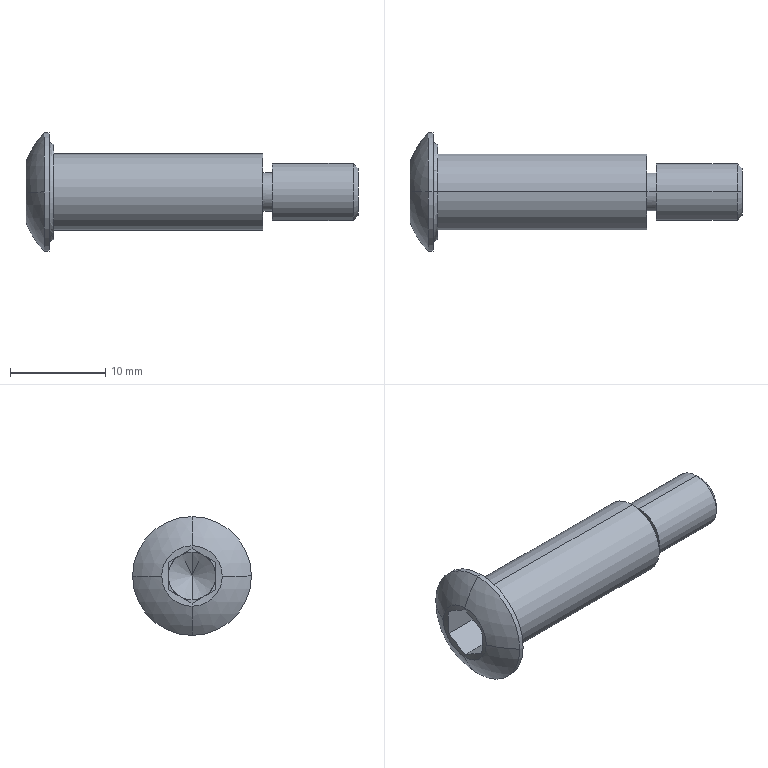Part | STEP file | 101000007750 | 1 solid | 39 faces | box 34.924 x 12.5 x 12.5 mm | volume 1534 mm3 | plane 17 | cylinder 10 | cone 6 | sphere 4 | torus 2 | commonest cylinder face diameters 4 x2 5 x2 6 x2 8 x2 12.5 x2
STEP:
#1=CARTESIAN_POINT('',(3.,0.,-5.5));
#2=VERTEX_POINT('',#1);
#3=CARTESIAN_POINT('',(3.,0.,5.5));
#4=VERTEX_POINT('',#3);
#5=CARTESIAN_POINT('',(3.,0.,0.));
#6=DIRECTION('',(-1.,0.,0.));
#7=AXIS2_PLACEMENT_3D('',#5,#6,$);
#8=CIRCLE('',#7,5.5);
#9=EDGE_CURVE('',#2,#4,#8,.T.);
#10=ORIENTED_EDGE('',*,*,#9,.F.);
#11=CARTESIAN_POINT('',(3.5,0.,-5.));
#12=VERTEX_POINT('',#11);
#13=CARTESIAN_POINT('',(3.5,0.,-5.5));
#14=DIRECTION('',(0.,1.,0.));
#15=AXIS2_PLACEMENT_3D('',#13,#14,$);
#16=CIRCLE('',#15,0.5);
#17=EDGE_CURVE('',#2,#12,#16,.T.);
#18=ORIENTED_EDGE('',*,*,#17,.T.);
#19=CARTESIAN_POINT('',(3.5,0.,5.));
#20=VERTEX_POINT('',#19);
#21=CARTESIAN_POINT('',(3.5,0.,0.));
#22=DIRECTION('',(-1.,0.,0.));
#23=AXIS2_PLACEMENT_3D('',#21,#22,$);
#24=CIRCLE('',#23,5.);
#25=EDGE_CURVE('',#12,#20,#24,.T.);
#26=ORIENTED_EDGE('',*,*,#25,.T.);
#27=CARTESIAN_POINT('',(3.5,0.,5.5));
#28=DIRECTION('',(0.,-1.,0.));
#29=AXIS2_PLACEMENT_3D('',#27,#28,$);
#30=CIRCLE('',#29,0.5);
#31=EDGE_CURVE('',#4,#20,#30,.T.);
#32=ORIENTED_EDGE('',*,*,#31,.F.);
#33=EDGE_LOOP('',(#10,#18,#26,#32));
#34=FACE_OUTER_BOUND('',#33,.T.);
#35=CARTESIAN_POINT('',(3.5,0.,0.));
#36=DIRECTION('',(-1.,0.,0.));
#37=DIRECTION('',(0.,0.,-1.));
#38=AXIS2_PLACEMENT_3D('',#35,#36,#37);
#39=TOROIDAL_SURFACE('',#38,5.5,0.5);
#40=ADVANCED_FACE('',(#34),#39,.F.);
#41=CARTESIAN_POINT('',(3.,0.,6.25));
#42=VERTEX_POINT('',#41);
#43=CARTESIAN_POINT('',(3.,0.,-6.25));
#44=VERTEX_POINT('',#43);
#45=CARTESIAN_POINT('',(3.,0.,0.));
#46=DIRECTION('',(-1.,0.,0.));
#47=AXIS2_PLACEMENT_3D('',#45,#46,$);
#48=CIRCLE('',#47,6.25);
#49=EDGE_CURVE('',#42,#44,#48,.T.);
#50=ORIENTED_EDGE('',*,*,#49,.F.);
#51=CARTESIAN_POINT('',(3.,0.,0.));
#52=DIRECTION('',(-1.,0.,0.));
#53=AXIS2_PLACEMENT_3D('',#51,#52,$);
#54=CIRCLE('',#53,6.25);
#55=EDGE_CURVE('',#44,#42,#54,.T.);
#56=ORIENTED_EDGE('',*,*,#55,.F.);
#57=EDGE_LOOP('',(#50,#56));
#58=FACE_OUTER_BOUND('',#57,.T.);
#59=CARTESIAN_POINT('',(3.,0.,0.));
#60=DIRECTION('',(-1.,0.,0.));
#61=AXIS2_PLACEMENT_3D('',#59,#60,$);
#62=CIRCLE('',#61,5.5);
#63=EDGE_CURVE('',#4,#2,#62,.T.);
#64=ORIENTED_EDGE('',*,*,#63,.T.);
#65=ORIENTED_EDGE('',*,*,#9,.T.);
#66=EDGE_LOOP('',(#64,#65));
#67=FACE_BOUND('',#66,.T.);
#68=CARTESIAN_POINT('',(3.,6.25,0.));
#69=DIRECTION('',(-1.,0.,0.));
#70=DIRECTION('',(0.,0.,1.));
#71=AXIS2_PLACEMENT_3D('',#68,#69,#70);
#72=PLANE('',#71);
#73=ADVANCED_FACE('',(#58,#67),#72,.F.);
#74=ORIENTED_EDGE('',*,*,#17,.F.);
#75=ORIENTED_EDGE('',*,*,#63,.F.);
#76=ORIENTED_EDGE('',*,*,#31,.T.);
#77=CARTESIAN_POINT('',(3.5,0.,0.));
#78=DIRECTION('',(-1.,0.,0.));
#79=AXIS2_PLACEMENT_3D('',#77,#78,$);
#80=CIRCLE('',#79,5.);
#81=EDGE_CURVE('',#20,#12,#80,.T.);
#82=ORIENTED_EDGE('',*,*,#81,.T.);
#83=EDGE_LOOP('',(#74,#75,#76,#82));
#84=FACE_OUTER_BOUND('',#83,.T.);
#85=CARTESIAN_POINT('',(3.5,0.,0.));
#86=DIRECTION('',(-1.,0.,0.));
#87=DIRECTION('',(0.,0.,1.));
#88=AXIS2_PLACEMENT_3D('',#85,#86,#87);
#89=TOROIDAL_SURFACE('',#88,5.5,0.5);
#90=ADVANCED_FACE('',(#84),#89,.F.);
#91=ORIENTED_EDGE('',*,*,#81,.F.);
#92=ORIENTED_EDGE('',*,*,#25,.F.);
#93=EDGE_LOOP('',(#91,#92));
#94=FACE_OUTER_BOUND('',#93,.T.);
#95=CARTESIAN_POINT('',(3.5,0.,4.));
#96=VERTEX_POINT('',#95);
#97=CARTESIAN_POINT('',(3.5,0.,-4.));
#98=VERTEX_POINT('',#97);
#99=CARTESIAN_POINT('',(3.5,0.,0.));
#100=DIRECTION('',(-1.,0.,0.));
#101=AXIS2_PLACEMENT_3D('',#99,#100,$);
#102=CIRCLE('',#101,4.);
#103=EDGE_CURVE('',#96,#98,#102,.T.);
#104=ORIENTED_EDGE('',*,*,#103,.T.);
#105=CARTESIAN_POINT('',(3.5,0.,0.));
#106=DIRECTION('',(-1.,0.,0.));
#107=AXIS2_PLACEMENT_3D('',#105,#106,$);
#108=CIRCLE('',#107,4.);
#109=EDGE_CURVE('',#98,#96,#108,.T.);
#110=ORIENTED_EDGE('',*,*,#109,.T.);
#111=EDGE_LOOP('',(#104,#110));
#112=FACE_BOUND('',#111,.T.);
#113=CARTESIAN_POINT('',(3.5,5.,0.));
#114=DIRECTION('',(-1.,0.,0.));
#115=DIRECTION('',(0.,0.,1.));
#116=AXIS2_PLACEMENT_3D('',#113,#114,#115);
#117=PLANE('',#116);
#118=ADVANCED_FACE('',(#94,#112),#117,.F.);
#119=ORIENTED_EDGE('',*,*,#49,.T.);
#120=CARTESIAN_POINT('',(2.5,0.,-6.25));
#121=VERTEX_POINT('',#120);
#122=CARTESIAN_POINT('',(0.,0.,-6.25));
#123=DIRECTION('',(-1.,0.,0.));
#124=VECTOR('',#123,1.);
#125=LINE('',#122,#124);
#126=EDGE_CURVE('',#44,#121,#125,.T.);
#127=ORIENTED_EDGE('',*,*,#126,.T.);
#128=CARTESIAN_POINT('',(2.5,6.25,0.));
#129=VERTEX_POINT('',#128);
#130=CARTESIAN_POINT('',(2.5,0.,0.));
#131=DIRECTION('',(-1.,0.,0.));
#132=AXIS2_PLACEMENT_3D('',#130,#131,$);
#133=CIRCLE('',#132,6.25);
#134=EDGE_CURVE('',#129,#121,#133,.T.);
#135=ORIENTED_EDGE('',*,*,#134,.F.);
#136=CARTESIAN_POINT('',(2.5,0.,6.25));
#137=VERTEX_POINT('',#136);
#138=CARTESIAN_POINT('',(2.5,0.,0.));
#139=DIRECTION('',(-1.,0.,0.));
#140=AXIS2_PLACEMENT_3D('',#138,#139,$);
#141=CIRCLE('',#140,6.25);
#142=EDGE_CURVE('',#137,#129,#141,.T.);
#143=ORIENTED_EDGE('',*,*,#142,.F.);
#144=CARTESIAN_POINT('',(0.,0.,6.25));
#145=DIRECTION('',(-1.,0.,0.));
#146=VECTOR('',#145,1.);
#147=LINE('',#144,#146);
#148=EDGE_CURVE('',#42,#137,#147,.T.);
#149=ORIENTED_EDGE('',*,*,#148,.F.);
#150=EDGE_LOOP('',(#119,#127,#135,#143,#149));
#151=FACE_OUTER_BOUND('',#150,.T.);
#152=CARTESIAN_POINT('',(0.,0.,0.));
#153=DIRECTION('',(-1.,0.,0.));
#154=DIRECTION('',(0.,0.,1.));
#155=AXIS2_PLACEMENT_3D('',#152,#153,#154);
#156=CYLINDRICAL_SURFACE('',#155,6.25);
#157=ADVANCED_FACE('',(#151),#156,.T.);
#158=ORIENTED_EDGE('',*,*,#126,.F.);
#159=ORIENTED_EDGE('',*,*,#55,.T.);
#160=ORIENTED_EDGE('',*,*,#148,.T.);
#161=CARTESIAN_POINT('',(2.5,-6.25,0.));
#162=VERTEX_POINT('',#161);
#163=CARTESIAN_POINT('',(2.5,0.,0.));
#164=DIRECTION('',(-1.,0.,0.));
#165=AXIS2_PLACEMENT_3D('',#163,#164,$);
#166=CIRCLE('',#165,6.25);
#167=EDGE_CURVE('',#162,#137,#166,.T.);
#168=ORIENTED_EDGE('',*,*,#167,.F.);
#169=CARTESIAN_POINT('',(2.5,0.,0.));
#170=DIRECTION('',(-1.,0.,0.));
#171=AXIS2_PLACEMENT_3D('',#169,#170,$);
#172=CIRCLE('',#171,6.25);
#173=EDGE_CURVE('',#121,#162,#172,.T.);
#174=ORIENTED_EDGE('',*,*,#173,.F.);
#175=EDGE_LOOP('',(#158,#159,#160,#168,#174));
#176=FACE_OUTER_BOUND('',#175,.T.);
#177=CARTESIAN_POINT('',(0.,0.,0.));
#178=DIRECTION('',(-1.,0.,0.));
#179=DIRECTION('',(0.,0.,-1.));
#180=AXIS2_PLACEMENT_3D('',#177,#178,#179);
#181=CYLINDRICAL_SURFACE('',#180,6.25);
#182=ADVANCED_FACE('',(#176),#181,.T.);
#183=CARTESIAN_POINT('',(25.5,0.,4.));
#184=VERTEX_POINT('',#183);
#185=CARTESIAN_POINT('',(25.5,0.,-4.));
#186=VERTEX_POINT('',#185);
#187=CARTESIAN_POINT('',(25.5,0.,0.));
#188=DIRECTION('',(-1.,0.,0.));
#189=AXIS2_PLACEMENT_3D('',#187,#188,$);
#190=CIRCLE('',#189,4.);
#191=EDGE_CURVE('',#184,#186,#190,.T.);
#192=ORIENTED_EDGE('',*,*,#191,.T.);
#193=CARTESIAN_POINT('',(0.,0.,-4.));
#194=DIRECTION('',(-1.,0.,0.));
#195=VECTOR('',#194,1.);
#196=LINE('',#193,#195);
#197=EDGE_CURVE('',#186,#98,#196,.T.);
#198=ORIENTED_EDGE('',*,*,#197,.T.);
#199=ORIENTED_EDGE('',*,*,#103,.F.);
#200=CARTESIAN_POINT('',(0.,0.,4.));
#201=DIRECTION('',(-1.,0.,0.));
#202=VECTOR('',#201,1.);
#203=LINE('',#200,#202);
#204=EDGE_CURVE('',#184,#96,#203,.T.);
#205=ORIENTED_EDGE('',*,*,#204,.F.);
#206=EDGE_LOOP('',(#192,#198,#199,#205));
#207=FACE_OUTER_BOUND('',#206,.T.);
#208=CARTESIAN_POINT('',(0.,0.,0.));
#209=DIRECTION('',(-1.,0.,0.));
#210=DIRECTION('',(0.,0.,1.));
#211=AXIS2_PLACEMENT_3D('',#208,#209,#210);
#212=CYLINDRICAL_SURFACE('',#211,4.);
#213=ADVANCED_FACE('',(#207),#212,.T.);
#214=ORIENTED_EDGE('',*,*,#197,.F.);
#215=CARTESIAN_POINT('',(25.5,0.,0.));
#216=DIRECTION('',(-1.,0.,0.));
#217=AXIS2_PLACEMENT_3D('',#215,#216,$);
#218=CIRCLE('',#217,4.);
#219=EDGE_CURVE('',#186,#184,#218,.T.);
#220=ORIENTED_EDGE('',*,*,#219,.T.);
#221=ORIENTED_EDGE('',*,*,#204,.T.);
#222=ORIENTED_EDGE('',*,*,#109,.F.);
#223=EDGE_LOOP('',(#214,#220,#221,#222));
#224=FACE_OUTER_BOUND('',#223,.T.);
#225=CARTESIAN_POINT('',(0.,0.,0.));
#226=DIRECTION('',(-1.,0.,0.));
#227=DIRECTION('',(0.,0.,-1.));
#228=AXIS2_PLACEMENT_3D('',#225,#226,#227);
#229=CYLINDRICAL_SURFACE('',#228,4.);
#230=ADVANCED_FACE('',(#224),#229,.T.);
#231=CARTESIAN_POINT('',(0.5761,0.,-3.18));
#232=VERTEX_POINT('',#231);
#233=CARTESIAN_POINT('',(9.062,0.,0.));
#234=DIRECTION('',(0.,-1.,0.));
#235=AXIS2_PLACEMENT_3D('',#233,#234,$);
#236=CIRCLE('',#235,9.062);
#237=EDGE_CURVE('',#232,#121,#236,.T.);
#238=ORIENTED_EDGE('',*,*,#237,.F.);
#239=CARTESIAN_POINT('',(0.5761,3.18,0.));
#240=VERTEX_POINT('',#239);
#241=CARTESIAN_POINT('',(0.5761,3.18,0.));
#242=CARTESIAN_POINT('',(0.5761,3.18,-1.011));
#243=CARTESIAN_POINT('',(0.5761,2.782,-2.028));
#244=CARTESIAN_POINT('',(0.5761,1.955,-2.812));
#245=CARTESIAN_POINT('',(0.5761,0.9776,-3.18));
#246=CARTESIAN_POINT('',(0.5761,0.,-3.18));
#247=B_SPLINE_CURVE_WITH_KNOTS('',5,(#241,#242,#243,#244,#245,#246),.UNSPECIFIED.,.F.,.U.,(6,6),(0.,7.151),.UNSPECIFIED.);
#248=EDGE_CURVE('',#240,#232,#247,.T.);
#249=ORIENTED_EDGE('',*,*,#248,.F.);
#250=CARTESIAN_POINT('',(9.062,0.,0.));
#251=DIRECTION('',(0.,0.,-1.));
#252=AXIS2_PLACEMENT_3D('',#250,#251,$);
#253=CIRCLE('',#252,9.062);
#254=EDGE_CURVE('',#129,#240,#253,.F.);
#255=ORIENTED_EDGE('',*,*,#254,.F.);
#256=ORIENTED_EDGE('',*,*,#134,.T.);
#257=EDGE_LOOP('',(#238,#249,#255,#256));
#258=FACE_OUTER_BOUND('',#257,.T.);
#259=CARTESIAN_POINT('',(9.062,0.,0.));
#260=DIRECTION('',(0.,0.,-1.));
#261=DIRECTION('',(-1.,0.,0.));
#262=AXIS2_PLACEMENT_3D('',#259,#260,#261);
#263=SPHERICAL_SURFACE('',#262,9.062);
#264=ADVANCED_FACE('',(#258),#263,.T.);
#265=CARTESIAN_POINT('',(0.5761,0.,3.18));
#266=VERTEX_POINT('',#265);
#267=CARTESIAN_POINT('',(9.062,0.,0.));
#268=DIRECTION('',(0.,-1.,0.));
#269=AXIS2_PLACEMENT_3D('',#267,#268,$);
#270=CIRCLE('',#269,9.062);
#271=EDGE_CURVE('',#137,#266,#270,.T.);
#272=ORIENTED_EDGE('',*,*,#271,.F.);
#273=ORIENTED_EDGE('',*,*,#142,.T.);
#274=ORIENTED_EDGE('',*,*,#254,.T.);
#275=CARTESIAN_POINT('',(0.5761,0.,3.18));
#276=CARTESIAN_POINT('',(0.5761,0.9776,3.18));
#277=CARTESIAN_POINT('',(0.5761,1.955,2.812));
#278=CARTESIAN_POINT('',(0.5761,2.782,2.028));
#279=CARTESIAN_POINT('',(0.5761,3.18,1.011));
#280=CARTESIAN_POINT('',(0.5761,3.18,0.));
#281=B_SPLINE_CURVE_WITH_KNOTS('',5,(#275,#276,#277,#278,#279,#280),.UNSPECIFIED.,.F.,.U.,(6,6),(0.,7.151),.UNSPECIFIED.);
#282=EDGE_CURVE('',#266,#240,#281,.T.);
#283=ORIENTED_EDGE('',*,*,#282,.F.);
#284=EDGE_LOOP('',(#272,#273,#274,#283));
#285=FACE_OUTER_BOUND('',#284,.T.);
#286=CARTESIAN_POINT('',(9.062,0.,0.));
#287=DIRECTION('',(0.,0.,-1.));
#288=DIRECTION('',(-1.,0.,0.));
#289=AXIS2_PLACEMENT_3D('',#286,#287,#288);
#290=SPHERICAL_SURFACE('',#289,9.062);
#291=ADVANCED_FACE('',(#285),#290,.T.);
#292=ORIENTED_EDGE('',*,*,#271,.T.);
#293=CARTESIAN_POINT('',(0.5761,-3.18,0.));
#294=VERTEX_POINT('',#293);
#295=CARTESIAN_POINT('',(0.5761,-3.18,0.));
#296=CARTESIAN_POINT('',(0.5761,-3.18,1.011));
#297=CARTESIAN_POINT('',(0.5761,-2.782,2.028));
#298=CARTESIAN_POINT('',(0.5761,-1.955,2.812));
#299=CARTESIAN_POINT('',(0.5761,-0.9776,3.18));
#300=CARTESIAN_POINT('',(0.5761,0.,3.18));
#301=B_SPLINE_CURVE_WITH_KNOTS('',5,(#295,#296,#297,#298,#299,#300),.UNSPECIFIED.,.F.,.U.,(6,6),(0.,7.151),.UNSPECIFIED.);
#302=EDGE_CURVE('',#294,#266,#301,.T.);
#303=ORIENTED_EDGE('',*,*,#302,.F.);
#304=CARTESIAN_POINT('',(9.062,0.,0.));
#305=DIRECTION('',(0.,0.,-1.));
#306=AXIS2_PLACEMENT_3D('',#304,#305,$);
#307=CIRCLE('',#306,9.062);
#308=EDGE_CURVE('',#162,#294,#307,.T.);
#309=ORIENTED_EDGE('',*,*,#308,.F.);
#310=ORIENTED_EDGE('',*,*,#167,.T.);
#311=EDGE_LOOP('',(#292,#303,#309,#310));
#312=FACE_OUTER_BOUND('',#311,.T.);
#313=CARTESIAN_POINT('',(9.062,0.,0.));
#314=DIRECTION('',(0.,0.,-1.));
#315=DIRECTION('',(0.,-1.,0.));
#316=AXIS2_PLACEMENT_3D('',#313,#314,#315);
#317=SPHERICAL_SURFACE('',#316,9.062);
#318=ADVANCED_FACE('',(#312),#317,.T.);
#319=ORIENTED_EDGE('',*,*,#237,.T.);
#320=ORIENTED_EDGE('',*,*,#173,.T.);
#321=ORIENTED_EDGE('',*,*,#308,.T.);
#322=CARTESIAN_POINT('',(0.5761,0.,-3.18));
#323=CARTESIAN_POINT('',(0.5761,-0.9776,-3.18));
#324=CARTESIAN_POINT('',(0.5761,-1.955,-2.812));
#325=CARTESIAN_POINT('',(0.5761,-2.782,-2.028));
#326=CARTESIAN_POINT('',(0.5761,-3.18,-1.011));
#327=CARTESIAN_POINT('',(0.5761,-3.18,0.));
#328=B_SPLINE_CURVE_WITH_KNOTS('',5,(#322,#323,#324,#325,#326,#327),.UNSPECIFIED.,.F.,.U.,(6,6),(0.,7.151),.UNSPECIFIED.);
#329=EDGE_CURVE('',#232,#294,#328,.T.);
#330=ORIENTED_EDGE('',*,*,#329,.F.);
#331=EDGE_LOOP('',(#319,#320,#321,#330));
#332=FACE_OUTER_BOUND('',#331,.T.);
#333=CARTESIAN_POINT('',(9.062,0.,0.));
#334=DIRECTION('',(0.,0.,-1.));
#335=DIRECTION('',(0.,-1.,0.));
#336=AXIS2_PLACEMENT_3D('',#333,#334,#335);
#337=SPHERICAL_SURFACE('',#336,9.062);
#338=ADVANCED_FACE('',(#332),#337,.T.);
#339=ORIENTED_EDGE('',*,*,#191,.F.);
#340=ORIENTED_EDGE('',*,*,#219,.F.);
#341=EDGE_LOOP('',(#339,#340));
#342=FACE_OUTER_BOUND('',#341,.T.);
#343=CARTESIAN_POINT('',(25.5,0.,-2.));
#344=VERTEX_POINT('',#343);
#345=CARTESIAN_POINT('',(25.5,0.,2.));
#346=VERTEX_POINT('',#345);
#347=CARTESIAN_POINT('',(25.5,0.,-2.));
#348=CARTESIAN_POINT('',(25.5,0.2078,-2.));
#349=CARTESIAN_POINT('',(25.5,0.4157,-1.973));
#350=CARTESIAN_POINT('',(25.5,0.6189,-1.919));
#351=CARTESIAN_POINT('',(25.5,1.006,-1.759));
#352=CARTESIAN_POINT('',(25.5,1.341,-1.506));
#353=CARTESIAN_POINT('',(25.5,1.49,-1.358));
#354=CARTESIAN_POINT('',(25.5,1.747,-1.027));
#355=CARTESIAN_POINT('',(25.5,1.911,-0.6418));
#356=CARTESIAN_POINT('',(25.5,1.968,-0.4392));
#357=CARTESIAN_POINT('',(25.5,2.027,-0.02422));
#358=CARTESIAN_POINT('',(25.5,1.978,0.3921));
#359=CARTESIAN_POINT('',(25.5,1.926,0.5959));
#360=CARTESIAN_POINT('',(25.5,1.771,0.9854));
#361=CARTESIAN_POINT('',(25.5,1.522,1.322));
#362=CARTESIAN_POINT('',(25.5,1.376,1.474));
#363=CARTESIAN_POINT('',(25.5,1.048,1.735));
#364=CARTESIAN_POINT('',(25.5,0.6646,1.904));
#365=CARTESIAN_POINT('',(25.5,0.4627,1.963));
#366=CARTESIAN_POINT('',(25.5,0.2461,1.996));
#367=CARTESIAN_POINT('',(25.5,0.02868,2.));
#368=CARTESIAN_POINT('',(25.5,0.01912,2.));
#369=CARTESIAN_POINT('',(25.5,0.00956,2.));
#370=CARTESIAN_POINT('',(25.5,0.,2.));
#371=B_SPLINE_CURVE_WITH_KNOTS('',5,(#347,#348,#349,#350,#351,#352,#353,#354,#355,#356,#357,#358,#359,#360,#361,#362,#363,#364,#365,#366,#367,#368,#369,#370),.UNSPECIFIED.,.F.,.U.,(6,3,3,3,3,3,3,6),(0.,1.47,2.939,4.409,5.879,7.348,8.818,8.886),.UNSPECIFIED.);
#372=EDGE_CURVE('',#344,#346,#371,.T.);
#373=ORIENTED_EDGE('',*,*,#372,.F.);
#374=CARTESIAN_POINT('',(25.5,0.,2.));
#375=CARTESIAN_POINT('',(25.5,-0.2078,2.));
#376=CARTESIAN_POINT('',(25.5,-0.4157,1.973));
#377=CARTESIAN_POINT('',(25.5,-0.6189,1.919));
#378=CARTESIAN_POINT('',(25.5,-1.006,1.759));
#379=CARTESIAN_POINT('',(25.5,-1.341,1.506));
#380=CARTESIAN_POINT('',(25.5,-1.49,1.358));
#381=CARTESIAN_POINT('',(25.5,-1.747,1.027));
#382=CARTESIAN_POINT('',(25.5,-1.911,0.6418));
#383=CARTESIAN_POINT('',(25.5,-1.968,0.4392));
#384=CARTESIAN_POINT('',(25.5,-2.027,0.02422));
#385=CARTESIAN_POINT('',(25.5,-1.978,-0.3921));
#386=CARTESIAN_POINT('',(25.5,-1.926,-0.5959));
#387=CARTESIAN_POINT('',(25.5,-1.771,-0.9854));
#388=CARTESIAN_POINT('',(25.5,-1.522,-1.322));
#389=CARTESIAN_POINT('',(25.5,-1.376,-1.474));
#390=CARTESIAN_POINT('',(25.5,-1.048,-1.735));
#391=CARTESIAN_POINT('',(25.5,-0.6646,-1.904));
#392=CARTESIAN_POINT('',(25.5,-0.4627,-1.963));
#393=CARTESIAN_POINT('',(25.5,-0.2461,-1.996));
#394=CARTESIAN_POINT('',(25.5,-0.02868,-2.));
#395=CARTESIAN_POINT('',(25.5,-0.01912,-2.));
#396=CARTESIAN_POINT('',(25.5,-0.00956,-2.));
#397=CARTESIAN_POINT('',(25.5,0.,-2.));
#398=B_SPLINE_CURVE_WITH_KNOTS('',5,(#374,#375,#376,#377,#378,#379,#380,#381,#382,#383,#384,#385,#386,#387,#388,#389,#390,#391,#392,#393,#394,#395,#396,#397),.UNSPECIFIED.,.F.,.U.,(6,3,3,3,3,3,3,6),(0.,1.47,2.939,4.409,5.879,7.348,8.818,8.886),.UNSPECIFIED.);
#399=EDGE_CURVE('',#346,#344,#398,.T.);
#400=ORIENTED_EDGE('',*,*,#399,.F.);
#401=EDGE_LOOP('',(#373,#400));
#402=FACE_BOUND('',#401,.T.);
#403=CARTESIAN_POINT('',(25.5,4.,0.));
#404=DIRECTION('',(-1.,0.,0.));
#405=DIRECTION('',(0.,0.,1.));
#406=AXIS2_PLACEMENT_3D('',#403,#404,#405);
#407=PLANE('',#406);
#408=ADVANCED_FACE('',(#342,#402),#407,.F.);
#409=CARTESIAN_POINT('',(0.6151,0.,-2.887));
#410=VERTEX_POINT('',#409);
#411=CARTESIAN_POINT('',(-66580.86,0.,-499363.95));
#412=DIRECTION('',(-0.1322,0.,-0.9912));
#413=VECTOR('',#412,1.);
#414=LINE('',#411,#413);
#415=EDGE_CURVE('',#410,#232,#414,.T.);
#416=ORIENTED_EDGE('',*,*,#415,.F.);
#417=CARTESIAN_POINT('',(0.6151,2.5,-1.443));
#418=VERTEX_POINT('',#417);
#419=CARTESIAN_POINT('',(0.6151,2.5,-1.443));
#420=CARTESIAN_POINT('',(0.6617,1.895,-1.793));
#421=CARTESIAN_POINT('',(0.6741,1.472,-2.037));
#422=CARTESIAN_POINT('',(0.6743,1.029,-2.293));
#423=CARTESIAN_POINT('',(0.6617,0.6048,-2.538));
#424=CARTESIAN_POINT('',(0.6151,0.,-2.887));
#425=B_SPLINE_CURVE_WITH_KNOTS('',5,(#419,#420,#421,#422,#423,#424),.UNSPECIFIED.,.F.,.U.,(6,6),(0.,104.832),.UNSPECIFIED.);
#426=EDGE_CURVE('',#418,#410,#425,.T.);
#427=ORIENTED_EDGE('',*,*,#426,.F.);
#428=CARTESIAN_POINT('',(0.6151,2.5,1.443));
#429=VERTEX_POINT('',#428);
#430=CARTESIAN_POINT('',(0.6151,2.5,1.443));
#431=CARTESIAN_POINT('',(0.6617,2.5,0.745));
#432=CARTESIAN_POINT('',(0.6742,2.5,0.2567));
#433=CARTESIAN_POINT('',(0.6743,2.5,-0.2555));
#434=CARTESIAN_POINT('',(0.6617,2.5,-0.745));
#435=CARTESIAN_POINT('',(0.6151,2.5,-1.443));
#436=B_SPLINE_CURVE_WITH_KNOTS('',5,(#430,#431,#432,#433,#434,#435),.UNSPECIFIED.,.F.,.U.,(6,6),(0.,104.832),.UNSPECIFIED.);
#437=EDGE_CURVE('',#429,#418,#436,.T.);
#438=ORIENTED_EDGE('',*,*,#437,.F.);
#439=CARTESIAN_POINT('',(0.6151,0.,2.887));
#440=VERTEX_POINT('',#439);
#441=CARTESIAN_POINT('',(0.6151,0.,2.887));
#442=CARTESIAN_POINT('',(0.6617,0.6048,2.538));
#443=CARTESIAN_POINT('',(0.6741,1.028,2.293));
#444=CARTESIAN_POINT('',(0.6743,1.471,2.037));
#445=CARTESIAN_POINT('',(0.6617,1.895,1.793));
#446=CARTESIAN_POINT('',(0.6151,2.5,1.443));
#447=B_SPLINE_CURVE_WITH_KNOTS('',5,(#441,#442,#443,#444,#445,#446),.UNSPECIFIED.,.F.,.U.,(6,6),(0.,104.832),.UNSPECIFIED.);
#448=EDGE_CURVE('',#440,#429,#447,.T.);
#449=ORIENTED_EDGE('',*,*,#448,.F.);
#450=CARTESIAN_POINT('',(-66580.86,0.,499363.95));
#451=DIRECTION('',(-0.1322,0.,0.9912));
#452=VECTOR('',#451,1.);
#453=LINE('',#450,#452);
#454=EDGE_CURVE('',#440,#266,#453,.T.);
#455=ORIENTED_EDGE('',*,*,#454,.T.);
#456=ORIENTED_EDGE('',*,*,#282,.T.);
#457=ORIENTED_EDGE('',*,*,#248,.T.);
#458=EDGE_LOOP('',(#416,#427,#438,#449,#455,#456,#457));
#459=FACE_OUTER_BOUND('',#458,.T.);
#460=CARTESIAN_POINT('',(-999.,0.,0.));
#461=DIRECTION('',(-1.,0.,0.));
#462=DIRECTION('',(0.,0.,1.));
#463=AXIS2_PLACEMENT_3D('',#460,#461,#462);
#464=CONICAL_SURFACE('',#463,7500.,1.438);
#465=ADVANCED_FACE('',(#459),#464,.F.);
#466=CARTESIAN_POINT('',(0.6151,-2.5,-1.443));
#467=VERTEX_POINT('',#466);
#468=CARTESIAN_POINT('',(0.6151,0.,-2.887));
#469=CARTESIAN_POINT('',(0.6617,-0.6048,-2.538));
#470=CARTESIAN_POINT('',(0.6741,-1.028,-2.293));
#471=CARTESIAN_POINT('',(0.6743,-1.471,-2.037));
#472=CARTESIAN_POINT('',(0.6617,-1.895,-1.793));
#473=CARTESIAN_POINT('',(0.6151,-2.5,-1.443));
#474=B_SPLINE_CURVE_WITH_KNOTS('',5,(#468,#469,#470,#471,#472,#473),.UNSPECIFIED.,.F.,.U.,(6,6),(0.,104.832),.UNSPECIFIED.);
#475=EDGE_CURVE('',#410,#467,#474,.T.);
#476=ORIENTED_EDGE('',*,*,#475,.F.);
#477=ORIENTED_EDGE('',*,*,#415,.T.);
#478=ORIENTED_EDGE('',*,*,#329,.T.);
#479=ORIENTED_EDGE('',*,*,#302,.T.);
#480=ORIENTED_EDGE('',*,*,#454,.F.);
#481=CARTESIAN_POINT('',(0.6151,-2.5,1.443));
#482=VERTEX_POINT('',#481);
#483=CARTESIAN_POINT('',(0.6151,-2.5,1.443));
#484=CARTESIAN_POINT('',(0.6617,-1.895,1.793));
#485=CARTESIAN_POINT('',(0.6741,-1.472,2.037));
#486=CARTESIAN_POINT('',(0.6743,-1.029,2.293));
#487=CARTESIAN_POINT('',(0.6617,-0.6048,2.538));
#488=CARTESIAN_POINT('',(0.6151,0.,2.887));
#489=B_SPLINE_CURVE_WITH_KNOTS('',5,(#483,#484,#485,#486,#487,#488),.UNSPECIFIED.,.F.,.U.,(6,6),(0.,104.832),.UNSPECIFIED.);
#490=EDGE_CURVE('',#482,#440,#489,.T.);
#491=ORIENTED_EDGE('',*,*,#490,.F.);
#492=CARTESIAN_POINT('',(0.6151,-2.5,-1.443));
#493=CARTESIAN_POINT('',(0.6617,-2.5,-0.745));
#494=CARTESIAN_POINT('',(0.6741,-2.5,-0.2567));
#495=CARTESIAN_POINT('',(0.6743,-2.5,0.2555));
#496=CARTESIAN_POINT('',(0.6617,-2.5,0.745));
#497=CARTESIAN_POINT('',(0.6151,-2.5,1.443));
#498=B_SPLINE_CURVE_WITH_KNOTS('',5,(#492,#493,#494,#495,#496,#497),.UNSPECIFIED.,.F.,.U.,(6,6),(0.,104.833),.UNSPECIFIED.);
#499=EDGE_CURVE('',#467,#482,#498,.T.);
#500=ORIENTED_EDGE('',*,*,#499,.F.);
#501=EDGE_LOOP('',(#476,#477,#478,#479,#480,#491,#500));
#502=FACE_OUTER_BOUND('',#501,.T.);
#503=CARTESIAN_POINT('',(-999.,0.,0.));
#504=DIRECTION('',(-1.,0.,0.));
#505=DIRECTION('',(0.,0.,-1.));
#506=AXIS2_PLACEMENT_3D('',#503,#504,#505);
#507=CONICAL_SURFACE('',#506,7500.,1.438);
#508=ADVANCED_FACE('',(#502),#507,.F.);
#509=ORIENTED_EDGE('',*,*,#372,.T.);
#510=CARTESIAN_POINT('',(26.5,0.,2.));
#511=VERTEX_POINT('',#510);
#512=CARTESIAN_POINT('',(35.,0.,2.));
#513=DIRECTION('',(1.,0.,0.));
#514=VECTOR('',#513,1.);
#515=LINE('',#512,#514);
#516=EDGE_CURVE('',#346,#511,#515,.T.);
#517=ORIENTED_EDGE('',*,*,#516,.T.);
#518=CARTESIAN_POINT('',(26.5,0.,-2.));
#519=VERTEX_POINT('',#518);
#520=CARTESIAN_POINT('',(26.5,0.,0.));
#521=DIRECTION('',(1.,0.,0.));
#522=AXIS2_PLACEMENT_3D('',#520,#521,$);
#523=CIRCLE('',#522,2.);
#524=EDGE_CURVE('',#519,#511,#523,.T.);
#525=ORIENTED_EDGE('',*,*,#524,.F.);
#526=CARTESIAN_POINT('',(35.,0.,-2.));
#527=DIRECTION('',(1.,0.,0.));
#528=VECTOR('',#527,1.);
#529=LINE('',#526,#528);
#530=EDGE_CURVE('',#344,#519,#529,.T.);
#531=ORIENTED_EDGE('',*,*,#530,.F.);
#532=EDGE_LOOP('',(#509,#517,#525,#531));
#533=FACE_OUTER_BOUND('',#532,.T.);
#534=CARTESIAN_POINT('',(35.,0.,0.));
#535=DIRECTION('',(1.,0.,0.));
#536=DIRECTION('',(0.,0.,-1.));
#537=AXIS2_PLACEMENT_3D('',#534,#535,#536);
#538=CYLINDRICAL_SURFACE('',#537,2.);
#539=ADVANCED_FACE('',(#533),#538,.T.);
#540=ORIENTED_EDGE('',*,*,#516,.F.);
#541=ORIENTED_EDGE('',*,*,#399,.T.);
#542=ORIENTED_EDGE('',*,*,#530,.T.);
#543=CARTESIAN_POINT('',(26.5,0.,0.));
#544=DIRECTION('',(1.,0.,0.));
#545=AXIS2_PLACEMENT_3D('',#543,#544,$);
#546=CIRCLE('',#545,2.);
#547=EDGE_CURVE('',#511,#519,#546,.T.);
#548=ORIENTED_EDGE('',*,*,#547,.F.);
#549=EDGE_LOOP('',(#540,#541,#542,#548));
#550=FACE_OUTER_BOUND('',#549,.T.);
#551=CARTESIAN_POINT('',(35.,0.,0.));
#552=DIRECTION('',(1.,0.,0.));
#553=DIRECTION('',(0.,0.,1.));
#554=AXIS2_PLACEMENT_3D('',#551,#552,#553);
#555=CYLINDRICAL_SURFACE('',#554,2.);
#556=ADVANCED_FACE('',(#550),#555,.T.);
#557=CARTESIAN_POINT('',(4.3,0.,-2.887));
#558=VERTEX_POINT('',#557);
#559=CARTESIAN_POINT('',(4.3,1.25,-2.165));
#560=VERTEX_POINT('',#559);
#561=CARTESIAN_POINT('',(4.3,0.625,-2.526));
#562=DIRECTION('',(0.,0.866,0.5));
#563=VECTOR('',#562,1.);
#564=LINE('',#561,#563);
#565=EDGE_CURVE('',#558,#560,#564,.T.);
#566=ORIENTED_EDGE('',*,*,#565,.T.);
#567=CARTESIAN_POINT('',(4.3,2.5,-1.443));
#568=VERTEX_POINT('',#567);
#569=CARTESIAN_POINT('',(4.3,1.875,-1.804));
#570=DIRECTION('',(0.,0.866,0.5));
#571=VECTOR('',#570,1.);
#572=LINE('',#569,#571);
#573=EDGE_CURVE('',#560,#568,#572,.T.);
#574=ORIENTED_EDGE('',*,*,#573,.T.);
#575=CARTESIAN_POINT('',(2.458,2.5,-1.443));
#576=DIRECTION('',(-1.,0.,0.));
#577=VECTOR('',#576,1.);
#578=LINE('',#575,#577);
#579=EDGE_CURVE('',#568,#418,#578,.T.);
#580=ORIENTED_EDGE('',*,*,#579,.T.);
#581=ORIENTED_EDGE('',*,*,#426,.T.);
#582=CARTESIAN_POINT('',(2.458,0.,-2.887));
#583=DIRECTION('',(-1.,0.,0.));
#584=VECTOR('',#583,1.);
#585=LINE('',#582,#584);
#586=EDGE_CURVE('',#558,#410,#585,.T.);
#587=ORIENTED_EDGE('',*,*,#586,.F.);
#588=EDGE_LOOP('',(#566,#574,#580,#581,#587));
#589=FACE_OUTER_BOUND('',#588,.T.);
#590=CARTESIAN_POINT('',(4.3,0.,-2.887));
#591=DIRECTION('',(0.,-0.5,0.866));
#592=DIRECTION('',(0.,-0.866,-0.5));
#593=AXIS2_PLACEMENT_3D('',#590,#591,#592);
#594=PLANE('',#593);
#595=ADVANCED_FACE('',(#589),#594,.T.);
#596=CARTESIAN_POINT('',(4.3,2.5,0.));
#597=VERTEX_POINT('',#596);
#598=CARTESIAN_POINT('',(4.3,2.5,-0.7217));
#599=DIRECTION('',(0.,0.,1.));
#600=VECTOR('',#599,1.);
#601=LINE('',#598,#600);
#602=EDGE_CURVE('',#568,#597,#601,.T.);
#603=ORIENTED_EDGE('',*,*,#602,.T.);
#604=CARTESIAN_POINT('',(4.3,2.5,1.443));
#605=VERTEX_POINT('',#604);
#606=CARTESIAN_POINT('',(4.3,2.5,0.7217));
#607=DIRECTION('',(0.,0.,1.));
#608=VECTOR('',#607,1.);
#609=LINE('',#606,#608);
#610=EDGE_CURVE('',#597,#605,#609,.T.);
#611=ORIENTED_EDGE('',*,*,#610,.T.);
#612=CARTESIAN_POINT('',(2.458,2.5,1.443));
#613=DIRECTION('',(-1.,0.,0.));
#614=VECTOR('',#613,1.);
#615=LINE('',#612,#614);
#616=EDGE_CURVE('',#605,#429,#615,.T.);
#617=ORIENTED_EDGE('',*,*,#616,.T.);
#618=ORIENTED_EDGE('',*,*,#437,.T.);
#619=ORIENTED_EDGE('',*,*,#579,.F.);
#620=EDGE_LOOP('',(#603,#611,#617,#618,#619));
#621=FACE_OUTER_BOUND('',#620,.T.);
#622=CARTESIAN_POINT('',(4.3,2.5,-1.443));
#623=DIRECTION('',(0.,-1.,0.));
#624=DIRECTION('',(0.,0.,-1.));
#625=AXIS2_PLACEMENT_3D('',#622,#623,#624);
#626=PLANE('',#625);
#627=ADVANCED_FACE('',(#621),#626,.T.);
#628=CARTESIAN_POINT('',(4.3,1.25,2.165));
#629=VERTEX_POINT('',#628);
#630=CARTESIAN_POINT('',(4.3,1.875,1.804));
#631=DIRECTION('',(0.,-0.866,0.5));
#632=VECTOR('',#631,1.);
#633=LINE('',#630,#632);
#634=EDGE_CURVE('',#605,#629,#633,.T.);
#635=ORIENTED_EDGE('',*,*,#634,.T.);
#636=CARTESIAN_POINT('',(4.3,0.,2.887));
#637=VERTEX_POINT('',#636);
#638=CARTESIAN_POINT('',(4.3,0.625,2.526));
#639=DIRECTION('',(0.,-0.866,0.5));
#640=VECTOR('',#639,1.);
#641=LINE('',#638,#640);
#642=EDGE_CURVE('',#629,#637,#641,.T.);
#643=ORIENTED_EDGE('',*,*,#642,.T.);
#644=CARTESIAN_POINT('',(2.458,0.,2.887));
#645=DIRECTION('',(-1.,0.,0.));
#646=VECTOR('',#645,1.);
#647=LINE('',#644,#646);
#648=EDGE_CURVE('',#637,#440,#647,.T.);
#649=ORIENTED_EDGE('',*,*,#648,.T.);
#650=ORIENTED_EDGE('',*,*,#448,.T.);
#651=ORIENTED_EDGE('',*,*,#616,.F.);
#652=EDGE_LOOP('',(#635,#643,#649,#650,#651));
#653=FACE_OUTER_BOUND('',#652,.T.);
#654=CARTESIAN_POINT('',(4.3,2.5,1.443));
#655=DIRECTION('',(0.,-0.5,-0.866));
#656=DIRECTION('',(0.,0.866,-0.5));
#657=AXIS2_PLACEMENT_3D('',#654,#655,#656);
#658=PLANE('',#657);
#659=ADVANCED_FACE('',(#653),#658,.T.);
#660=CARTESIAN_POINT('',(4.3,-2.5,-1.443));
#661=VERTEX_POINT('',#660);
#662=CARTESIAN_POINT('',(4.3,-1.25,-2.165));
#663=VERTEX_POINT('',#662);
#664=CARTESIAN_POINT('',(4.3,-1.875,-1.804));
#665=DIRECTION('',(0.,0.866,-0.5));
#666=VECTOR('',#665,1.);
#667=LINE('',#664,#666);
#668=EDGE_CURVE('',#661,#663,#667,.T.);
#669=ORIENTED_EDGE('',*,*,#668,.T.);
#670=CARTESIAN_POINT('',(4.3,-0.625,-2.526));
#671=DIRECTION('',(0.,0.866,-0.5));
#672=VECTOR('',#671,1.);
#673=LINE('',#670,#672);
#674=EDGE_CURVE('',#663,#558,#673,.T.);
#675=ORIENTED_EDGE('',*,*,#674,.T.);
#676=ORIENTED_EDGE('',*,*,#586,.T.);
#677=ORIENTED_EDGE('',*,*,#475,.T.);
#678=CARTESIAN_POINT('',(2.458,-2.5,-1.443));
#679=DIRECTION('',(-1.,0.,0.));
#680=VECTOR('',#679,1.);
#681=LINE('',#678,#680);
#682=EDGE_CURVE('',#661,#467,#681,.T.);
#683=ORIENTED_EDGE('',*,*,#682,.F.);
#684=EDGE_LOOP('',(#669,#675,#676,#677,#683));
#685=FACE_OUTER_BOUND('',#684,.T.);
#686=CARTESIAN_POINT('',(4.3,-2.5,-1.443));
#687=DIRECTION('',(0.,0.5,0.866));
#688=DIRECTION('',(0.,-0.866,0.5));
#689=AXIS2_PLACEMENT_3D('',#686,#687,#688);
#690=PLANE('',#689);
#691=ADVANCED_FACE('',(#685),#690,.T.);
#692=CARTESIAN_POINT('',(4.3,-1.25,2.165));
#693=VERTEX_POINT('',#692);
#694=CARTESIAN_POINT('',(4.3,-0.625,2.526));
#695=DIRECTION('',(0.,-0.866,-0.5));
#696=VECTOR('',#695,1.);
#697=LINE('',#694,#696);
#698=EDGE_CURVE('',#637,#693,#697,.T.);
#699=ORIENTED_EDGE('',*,*,#698,.T.);
#700=CARTESIAN_POINT('',(4.3,-2.5,1.443));
#701=VERTEX_POINT('',#700);
#702=CARTESIAN_POINT('',(4.3,-1.875,1.804));
#703=DIRECTION('',(0.,-0.866,-0.5));
#704=VECTOR('',#703,1.);
#705=LINE('',#702,#704);
#706=EDGE_CURVE('',#693,#701,#705,.T.);
#707=ORIENTED_EDGE('',*,*,#706,.T.);
#708=CARTESIAN_POINT('',(2.458,-2.5,1.443));
#709=DIRECTION('',(-1.,0.,0.));
#710=VECTOR('',#709,1.);
#711=LINE('',#708,#710);
#712=EDGE_CURVE('',#701,#482,#711,.T.);
#713=ORIENTED_EDGE('',*,*,#712,.T.);
#714=ORIENTED_EDGE('',*,*,#490,.T.);
#715=ORIENTED_EDGE('',*,*,#648,.F.);
#716=EDGE_LOOP('',(#699,#707,#713,#714,#715));
#717=FACE_OUTER_BOUND('',#716,.T.);
#718=CARTESIAN_POINT('',(4.3,0.,2.887));
#719=DIRECTION('',(0.,0.5,-0.866));
#720=DIRECTION('',(0.,0.866,0.5));
#721=AXIS2_PLACEMENT_3D('',#718,#719,#720);
#722=PLANE('',#721);
#723=ADVANCED_FACE('',(#717),#722,.T.);
#724=CARTESIAN_POINT('',(4.3,-2.5,0.));
#725=VERTEX_POINT('',#724);
#726=CARTESIAN_POINT('',(4.3,-2.5,0.7217));
#727=DIRECTION('',(0.,0.,-1.));
#728=VECTOR('',#727,1.);
#729=LINE('',#726,#728);
#730=EDGE_CURVE('',#701,#725,#729,.T.);
#731=ORIENTED_EDGE('',*,*,#730,.T.);
#732=CARTESIAN_POINT('',(4.3,-2.5,-0.7217));
#733=DIRECTION('',(0.,0.,-1.));
#734=VECTOR('',#733,1.);
#735=LINE('',#732,#734);
#736=EDGE_CURVE('',#725,#661,#735,.T.);
#737=ORIENTED_EDGE('',*,*,#736,.T.);
#738=ORIENTED_EDGE('',*,*,#682,.T.);
#739=ORIENTED_EDGE('',*,*,#499,.T.);
#740=ORIENTED_EDGE('',*,*,#712,.F.);
#741=EDGE_LOOP('',(#731,#737,#738,#739,#740));
#742=FACE_OUTER_BOUND('',#741,.T.);
#743=CARTESIAN_POINT('',(4.3,-2.5,1.443));
#744=DIRECTION('',(0.,1.,0.));
#745=DIRECTION('',(0.,0.,1.));
#746=AXIS2_PLACEMENT_3D('',#743,#744,#745);
#747=PLANE('',#746);
#748=ADVANCED_FACE('',(#742),#747,.T.);
#749=CARTESIAN_POINT('',(26.5,0.,3.));
#750=VERTEX_POINT('',#749);
#751=CARTESIAN_POINT('',(26.5,0.,-3.));
#752=VERTEX_POINT('',#751);
#753=CARTESIAN_POINT('',(26.5,0.,0.));
#754=DIRECTION('',(-1.,0.,0.));
#755=AXIS2_PLACEMENT_3D('',#753,#754,$);
#756=CIRCLE('',#755,3.);
#757=EDGE_CURVE('',#750,#752,#756,.T.);
#758=ORIENTED_EDGE('',*,*,#757,.T.);
#759=CARTESIAN_POINT('',(26.5,0.,0.));
#760=DIRECTION('',(-1.,0.,0.));
#761=AXIS2_PLACEMENT_3D('',#759,#760,$);
#762=CIRCLE('',#761,3.);
#763=EDGE_CURVE('',#752,#750,#762,.T.);
#764=ORIENTED_EDGE('',*,*,#763,.T.);
#765=EDGE_LOOP('',(#758,#764));
#766=FACE_OUTER_BOUND('',#765,.T.);
#767=ORIENTED_EDGE('',*,*,#524,.T.);
#768=ORIENTED_EDGE('',*,*,#547,.T.);
#769=EDGE_LOOP('',(#767,#768));
#770=FACE_BOUND('',#769,.T.);
#771=CARTESIAN_POINT('',(26.5,-3.046,0.));
#772=DIRECTION('',(-1.,0.,0.));
#773=DIRECTION('',(0.,0.,1.));
#774=AXIS2_PLACEMENT_3D('',#771,#772,#773);
#775=PLANE('',#774);
#776=ADVANCED_FACE('',(#766,#770),#775,.T.);
#777=CARTESIAN_POINT('',(4.3,0.,-2.5));
#778=VERTEX_POINT('',#777);
#779=CARTESIAN_POINT('',(4.3,1.25,-2.165));
#780=CARTESIAN_POINT('',(4.3,1.023,-2.296));
#781=CARTESIAN_POINT('',(4.3,0.7794,-2.397));
#782=CARTESIAN_POINT('',(4.3,0.5236,-2.466));
#783=CARTESIAN_POINT('',(4.3,0.2618,-2.5));
#784=CARTESIAN_POINT('',(4.3,0.,-2.5));
#785=B_SPLINE_CURVE_WITH_KNOTS('',5,(#779,#780,#781,#782,#783,#784),.UNSPECIFIED.,.F.,.U.,(6,6),(0.,1.851),.UNSPECIFIED.);
#786=EDGE_CURVE('',#560,#778,#785,.T.);
#787=ORIENTED_EDGE('',*,*,#786,.F.);
#788=ORIENTED_EDGE('',*,*,#565,.F.);
#789=ORIENTED_EDGE('',*,*,#674,.F.);
#790=CARTESIAN_POINT('',(4.3,0.,-2.5));
#791=CARTESIAN_POINT('',(4.3,-0.2618,-2.5));
#792=CARTESIAN_POINT('',(4.3,-0.5236,-2.466));
#793=CARTESIAN_POINT('',(4.3,-0.7794,-2.397));
#794=CARTESIAN_POINT('',(4.3,-1.023,-2.296));
#795=CARTESIAN_POINT('',(4.3,-1.25,-2.165));
#796=B_SPLINE_CURVE_WITH_KNOTS('',5,(#790,#791,#792,#793,#794,#795),.UNSPECIFIED.,.F.,.U.,(6,6),(0.,1.851),.UNSPECIFIED.);
#797=EDGE_CURVE('',#778,#663,#796,.T.);
#798=ORIENTED_EDGE('',*,*,#797,.F.);
#799=EDGE_LOOP('',(#787,#788,#789,#798));
#800=FACE_OUTER_BOUND('',#799,.T.);
#801=CARTESIAN_POINT('',(4.3,0.,2.887));
#802=DIRECTION('',(1.,0.,0.));
#803=DIRECTION('',(0.,0.,-1.));
#804=AXIS2_PLACEMENT_3D('',#801,#802,#803);
#805=PLANE('',#804);
#806=ADVANCED_FACE('',(#800),#805,.F.);
#807=CARTESIAN_POINT('',(4.3,2.5,0.));
#808=CARTESIAN_POINT('',(4.3,2.5,-0.2324));
#809=CARTESIAN_POINT('',(4.3,2.473,-0.4648));
#810=CARTESIAN_POINT('',(4.3,2.419,-0.693));
#811=CARTESIAN_POINT('',(4.3,2.259,-1.133));
#812=CARTESIAN_POINT('',(4.3,2.002,-1.524));
#813=CARTESIAN_POINT('',(4.3,1.852,-1.704));
#814=CARTESIAN_POINT('',(4.3,1.639,-1.905));
#815=CARTESIAN_POINT('',(4.3,1.4,-2.072));
#816=CARTESIAN_POINT('',(4.3,1.351,-2.105));
#817=CARTESIAN_POINT('',(4.3,1.301,-2.136));
#818=CARTESIAN_POINT('',(4.3,1.25,-2.165));
#819=B_SPLINE_CURVE_WITH_KNOTS('',5,(#807,#808,#809,#810,#811,#812,#813,#814,#815,#816,#817,#818),.UNSPECIFIED.,.F.,.U.,(6,3,3,6),(0.,1.643,3.286,3.702),.UNSPECIFIED.);
#820=EDGE_CURVE('',#597,#560,#819,.T.);
#821=ORIENTED_EDGE('',*,*,#820,.F.);
#822=ORIENTED_EDGE('',*,*,#602,.F.);
#823=ORIENTED_EDGE('',*,*,#573,.F.);
#824=EDGE_LOOP('',(#821,#822,#823));
#825=FACE_OUTER_BOUND('',#824,.T.);
#826=CARTESIAN_POINT('',(4.3,0.,2.887));
#827=DIRECTION('',(1.,0.,0.));
#828=DIRECTION('',(0.,0.,-1.));
#829=AXIS2_PLACEMENT_3D('',#826,#827,#828);
#830=PLANE('',#829);
#831=ADVANCED_FACE('',(#825),#830,.F.);
#832=CARTESIAN_POINT('',(4.3,1.25,2.165));
#833=CARTESIAN_POINT('',(4.3,1.451,2.049));
#834=CARTESIAN_POINT('',(4.3,1.639,1.909));
#835=CARTESIAN_POINT('',(4.3,1.81,1.748));
#836=CARTESIAN_POINT('',(4.3,2.11,1.39));
#837=CARTESIAN_POINT('',(4.3,2.321,0.9722));
#838=CARTESIAN_POINT('',(4.3,2.401,0.7519));
#839=CARTESIAN_POINT('',(4.3,2.469,0.4667));
#840=CARTESIAN_POINT('',(4.3,2.495,0.1765));
#841=CARTESIAN_POINT('',(4.3,2.498,0.1176));
#842=CARTESIAN_POINT('',(4.3,2.5,0.05882));
#843=CARTESIAN_POINT('',(4.3,2.5,0.));
#844=B_SPLINE_CURVE_WITH_KNOTS('',5,(#832,#833,#834,#835,#836,#837,#838,#839,#840,#841,#842,#843),.UNSPECIFIED.,.F.,.U.,(6,3,3,6),(0.,1.643,3.286,3.702),.UNSPECIFIED.);
#845=EDGE_CURVE('',#629,#597,#844,.T.);
#846=ORIENTED_EDGE('',*,*,#845,.F.);
#847=ORIENTED_EDGE('',*,*,#634,.F.);
#848=ORIENTED_EDGE('',*,*,#610,.F.);
#849=EDGE_LOOP('',(#846,#847,#848));
#850=FACE_OUTER_BOUND('',#849,.T.);
#851=CARTESIAN_POINT('',(4.3,0.,2.887));
#852=DIRECTION('',(1.,0.,0.));
#853=DIRECTION('',(0.,0.,-1.));
#854=AXIS2_PLACEMENT_3D('',#851,#852,#853);
#855=PLANE('',#854);
#856=ADVANCED_FACE('',(#850),#855,.F.);
#857=CARTESIAN_POINT('',(4.3,0.,2.5));
#858=VERTEX_POINT('',#857);
#859=CARTESIAN_POINT('',(4.3,-1.25,2.165));
#860=CARTESIAN_POINT('',(4.3,-1.023,2.296));
#861=CARTESIAN_POINT('',(4.3,-0.7794,2.397));
#862=CARTESIAN_POINT('',(4.3,-0.5236,2.466));
#863=CARTESIAN_POINT('',(4.3,-0.2618,2.5));
#864=CARTESIAN_POINT('',(4.3,0.,2.5));
#865=B_SPLINE_CURVE_WITH_KNOTS('',5,(#859,#860,#861,#862,#863,#864),.UNSPECIFIED.,.F.,.U.,(6,6),(0.,1.851),.UNSPECIFIED.);
#866=EDGE_CURVE('',#693,#858,#865,.T.);
#867=ORIENTED_EDGE('',*,*,#866,.F.);
#868=ORIENTED_EDGE('',*,*,#698,.F.);
#869=ORIENTED_EDGE('',*,*,#642,.F.);
#870=CARTESIAN_POINT('',(4.3,0.,2.5));
#871=CARTESIAN_POINT('',(4.3,0.2618,2.5));
#872=CARTESIAN_POINT('',(4.3,0.5236,2.466));
#873=CARTESIAN_POINT('',(4.3,0.7794,2.397));
#874=CARTESIAN_POINT('',(4.3,1.023,2.296));
#875=CARTESIAN_POINT('',(4.3,1.25,2.165));
#876=B_SPLINE_CURVE_WITH_KNOTS('',5,(#870,#871,#872,#873,#874,#875),.UNSPECIFIED.,.F.,.U.,(6,6),(0.,1.851),.UNSPECIFIED.);
#877=EDGE_CURVE('',#858,#629,#876,.T.);
#878=ORIENTED_EDGE('',*,*,#877,.F.);
#879=EDGE_LOOP('',(#867,#868,#869,#878));
#880=FACE_OUTER_BOUND('',#879,.T.);
#881=CARTESIAN_POINT('',(4.3,0.,2.887));
#882=DIRECTION('',(1.,0.,0.));
#883=DIRECTION('',(0.,0.,-1.));
#884=AXIS2_PLACEMENT_3D('',#881,#882,#883);
#885=PLANE('',#884);
#886=ADVANCED_FACE('',(#880),#885,.F.);
#887=CARTESIAN_POINT('',(4.3,-1.25,-2.165));
#888=CARTESIAN_POINT('',(4.3,-1.451,-2.049));
#889=CARTESIAN_POINT('',(4.3,-1.639,-1.909));
#890=CARTESIAN_POINT('',(4.3,-1.81,-1.748));
#891=CARTESIAN_POINT('',(4.3,-2.11,-1.39));
#892=CARTESIAN_POINT('',(4.3,-2.321,-0.9722));
#893=CARTESIAN_POINT('',(4.3,-2.401,-0.7519));
#894=CARTESIAN_POINT('',(4.3,-2.469,-0.4667));
#895=CARTESIAN_POINT('',(4.3,-2.495,-0.1765));
#896=CARTESIAN_POINT('',(4.3,-2.498,-0.1176));
#897=CARTESIAN_POINT('',(4.3,-2.5,-0.05882));
#898=CARTESIAN_POINT('',(4.3,-2.5,0.));
#899=B_SPLINE_CURVE_WITH_KNOTS('',5,(#887,#888,#889,#890,#891,#892,#893,#894,#895,#896,#897,#898),.UNSPECIFIED.,.F.,.U.,(6,3,3,6),(0.,1.643,3.286,3.702),.UNSPECIFIED.);
#900=EDGE_CURVE('',#663,#725,#899,.T.);
#901=ORIENTED_EDGE('',*,*,#900,.F.);
#902=ORIENTED_EDGE('',*,*,#668,.F.);
#903=ORIENTED_EDGE('',*,*,#736,.F.);
#904=EDGE_LOOP('',(#901,#902,#903));
#905=FACE_OUTER_BOUND('',#904,.T.);
#906=CARTESIAN_POINT('',(4.3,0.,2.887));
#907=DIRECTION('',(1.,0.,0.));
#908=DIRECTION('',(0.,0.,-1.));
#909=AXIS2_PLACEMENT_3D('',#906,#907,#908);
#910=PLANE('',#909);
#911=ADVANCED_FACE('',(#905),#910,.F.);
#912=CARTESIAN_POINT('',(4.3,-2.5,0.));
#913=CARTESIAN_POINT('',(4.3,-2.5,0.2324));
#914=CARTESIAN_POINT('',(4.3,-2.473,0.4648));
#915=CARTESIAN_POINT('',(4.3,-2.419,0.693));
#916=CARTESIAN_POINT('',(4.3,-2.259,1.133));
#917=CARTESIAN_POINT('',(4.3,-2.002,1.524));
#918=CARTESIAN_POINT('',(4.3,-1.852,1.704));
#919=CARTESIAN_POINT('',(4.3,-1.639,1.905));
#920=CARTESIAN_POINT('',(4.3,-1.4,2.072));
#921=CARTESIAN_POINT('',(4.3,-1.351,2.105));
#922=CARTESIAN_POINT('',(4.3,-1.301,2.136));
#923=CARTESIAN_POINT('',(4.3,-1.25,2.165));
#924=B_SPLINE_CURVE_WITH_KNOTS('',5,(#912,#913,#914,#915,#916,#917,#918,#919,#920,#921,#922,#923),.UNSPECIFIED.,.F.,.U.,(6,3,3,6),(0.,1.643,3.286,3.702),.UNSPECIFIED.);
#925=EDGE_CURVE('',#725,#693,#924,.T.);
#926=ORIENTED_EDGE('',*,*,#925,.F.);
#927=ORIENTED_EDGE('',*,*,#730,.F.);
#928=ORIENTED_EDGE('',*,*,#706,.F.);
#929=EDGE_LOOP('',(#926,#927,#928));
#930=FACE_OUTER_BOUND('',#929,.T.);
#931=CARTESIAN_POINT('',(4.3,0.,2.887));
#932=DIRECTION('',(1.,0.,0.));
#933=DIRECTION('',(0.,0.,-1.));
#934=AXIS2_PLACEMENT_3D('',#931,#932,#933);
#935=PLANE('',#934);
#936=ADVANCED_FACE('',(#930),#935,.F.);
#937=CARTESIAN_POINT('',(35.,0.,3.));
#938=VERTEX_POINT('',#937);
#939=CARTESIAN_POINT('',(35.,0.,-3.));
#940=VERTEX_POINT('',#939);
#941=CARTESIAN_POINT('',(35.,0.,0.));
#942=DIRECTION('',(-1.,0.,0.));
#943=AXIS2_PLACEMENT_3D('',#941,#942,$);
#944=CIRCLE('',#943,3.);
#945=EDGE_CURVE('',#938,#940,#944,.T.);
#946=ORIENTED_EDGE('',*,*,#945,.T.);
#947=CARTESIAN_POINT('',(35.5,0.,-3.));
#948=DIRECTION('',(-1.,0.,0.));
#949=VECTOR('',#948,1.);
#950=LINE('',#947,#949);
#951=EDGE_CURVE('',#940,#752,#950,.T.);
#952=ORIENTED_EDGE('',*,*,#951,.T.);
#953=ORIENTED_EDGE('',*,*,#757,.F.);
#954=CARTESIAN_POINT('',(35.5,0.,3.));
#955=DIRECTION('',(-1.,0.,0.));
#956=VECTOR('',#955,1.);
#957=LINE('',#954,#956);
#958=EDGE_CURVE('',#938,#750,#957,.T.);
#959=ORIENTED_EDGE('',*,*,#958,.F.);
#960=EDGE_LOOP('',(#946,#952,#953,#959));
#961=FACE_OUTER_BOUND('',#960,.T.);
#962=CARTESIAN_POINT('',(35.5,0.,0.));
#963=DIRECTION('',(-1.,0.,0.));
#964=DIRECTION('',(0.,0.,1.));
#965=AXIS2_PLACEMENT_3D('',#962,#963,#964);
#966=CYLINDRICAL_SURFACE('',#965,3.);
#967=ADVANCED_FACE('',(#961),#966,.T.);
#968=ORIENTED_EDGE('',*,*,#951,.F.);
#969=CARTESIAN_POINT('',(35.,0.,0.));
#970=DIRECTION('',(-1.,0.,0.));
#971=AXIS2_PLACEMENT_3D('',#969,#970,$);
#972=CIRCLE('',#971,3.);
#973=EDGE_CURVE('',#940,#938,#972,.T.);
#974=ORIENTED_EDGE('',*,*,#973,.T.);
#975=ORIENTED_EDGE('',*,*,#958,.T.);
#976=ORIENTED_EDGE('',*,*,#763,.F.);
#977=EDGE_LOOP('',(#968,#974,#975,#976));
#978=FACE_OUTER_BOUND('',#977,.T.);
#979=CARTESIAN_POINT('',(35.5,0.,0.));
#980=DIRECTION('',(-1.,0.,0.));
#981=DIRECTION('',(0.,0.,-1.));
#982=AXIS2_PLACEMENT_3D('',#979,#980,#981);
#983=CYLINDRICAL_SURFACE('',#982,3.);
#984=ADVANCED_FACE('',(#978),#983,.T.);
#985=CARTESIAN_POINT('',(4.326,0.,-2.5));
#986=VERTEX_POINT('',#985);
#987=CARTESIAN_POINT('',(0.,0.,-2.5));
#988=DIRECTION('',(-1.,0.,0.));
#989=VECTOR('',#988,1.);
#990=LINE('',#987,#989);
#991=EDGE_CURVE('',#986,#778,#990,.T.);
#992=ORIENTED_EDGE('',*,*,#991,.F.);
#993=CARTESIAN_POINT('',(4.326,0.,2.5));
#994=VERTEX_POINT('',#993);
#995=CARTESIAN_POINT('',(4.326,0.,2.5));
#996=CARTESIAN_POINT('',(4.326,0.7854,2.5));
#997=CARTESIAN_POINT('',(4.326,1.571,2.192));
#998=CARTESIAN_POINT('',(4.326,2.192,1.571));
#999=CARTESIAN_POINT('',(4.326,2.808,0.));
#1000=CARTESIAN_POINT('',(4.326,2.192,-1.571));
#1001=CARTESIAN_POINT('',(4.326,1.571,-2.192));
#1002=CARTESIAN_POINT('',(4.326,0.7854,-2.5));
#1003=CARTESIAN_POINT('',(4.326,0.,-2.5));
#1004=B_SPLINE_CURVE_WITH_KNOTS('',5,(#995,#996,#997,#998,#999,#1000,#1001,#1002,#1003),.UNSPECIFIED.,.F.,.U.,(6,3,6),(-3.927,0.,3.927),.UNSPECIFIED.);
#1005=EDGE_CURVE('',#994,#986,#1004,.T.);
#1006=ORIENTED_EDGE('',*,*,#1005,.F.);
#1007=CARTESIAN_POINT('',(0.,0.,2.5));
#1008=DIRECTION('',(-1.,0.,0.));
#1009=VECTOR('',#1008,1.);
#1010=LINE('',#1007,#1009);
#1011=EDGE_CURVE('',#994,#858,#1010,.T.);
#1012=ORIENTED_EDGE('',*,*,#1011,.T.);
#1013=ORIENTED_EDGE('',*,*,#877,.T.);
#1014=ORIENTED_EDGE('',*,*,#845,.T.);
#1015=ORIENTED_EDGE('',*,*,#820,.T.);
#1016=ORIENTED_EDGE('',*,*,#786,.T.);
#1017=EDGE_LOOP('',(#992,#1006,#1012,#1013,#1014,#1015,#1016));
#1018=FACE_OUTER_BOUND('',#1017,.T.);
#1019=CARTESIAN_POINT('',(0.,0.,0.));
#1020=DIRECTION('',(-1.,0.,0.));
#1021=DIRECTION('',(0.,0.,1.));
#1022=AXIS2_PLACEMENT_3D('',#1019,#1020,#1021);
#1023=CYLINDRICAL_SURFACE('',#1022,2.5);
#1024=ADVANCED_FACE('',(#1018),#1023,.F.);
#1025=CARTESIAN_POINT('',(4.326,0.,-2.5));
#1026=CARTESIAN_POINT('',(4.326,-0.7854,-2.5));
#1027=CARTESIAN_POINT('',(4.326,-1.571,-2.192));
#1028=CARTESIAN_POINT('',(4.326,-2.192,-1.571));
#1029=CARTESIAN_POINT('',(4.326,-2.808,0.));
#1030=CARTESIAN_POINT('',(4.326,-2.192,1.571));
#1031=CARTESIAN_POINT('',(4.326,-1.571,2.192));
#1032=CARTESIAN_POINT('',(4.326,-0.7854,2.5));
#1033=CARTESIAN_POINT('',(4.326,0.,2.5));
#1034=B_SPLINE_CURVE_WITH_KNOTS('',5,(#1025,#1026,#1027,#1028,#1029,#1030,#1031,#1032,#1033),.UNSPECIFIED.,.F.,.U.,(6,3,6),(-3.927,0.,3.927),.UNSPECIFIED.);
#1035=EDGE_CURVE('',#986,#994,#1034,.T.);
#1036=ORIENTED_EDGE('',*,*,#1035,.F.);
#1037=ORIENTED_EDGE('',*,*,#991,.T.);
#1038=ORIENTED_EDGE('',*,*,#797,.T.);
#1039=ORIENTED_EDGE('',*,*,#900,.T.);
#1040=ORIENTED_EDGE('',*,*,#925,.T.);
#1041=ORIENTED_EDGE('',*,*,#866,.T.);
#1042=ORIENTED_EDGE('',*,*,#1011,.F.);
#1043=EDGE_LOOP('',(#1036,#1037,#1038,#1039,#1040,#1041,#1042));
#1044=FACE_OUTER_BOUND('',#1043,.T.);
#1045=CARTESIAN_POINT('',(0.,0.,0.));
#1046=DIRECTION('',(-1.,0.,0.));
#1047=DIRECTION('',(0.,0.,-1.));
#1048=AXIS2_PLACEMENT_3D('',#1045,#1046,#1047);
#1049=CYLINDRICAL_SURFACE('',#1048,2.5);
#1050=ADVANCED_FACE('',(#1044),#1049,.F.);
#1051=CARTESIAN_POINT('',(35.5,0.,-2.5));
#1052=VERTEX_POINT('',#1051);
#1053=CARTESIAN_POINT('',(35.5,0.,2.5));
#1054=VERTEX_POINT('',#1053);
#1055=CARTESIAN_POINT('',(35.5,0.,0.));
#1056=DIRECTION('',(-1.,0.,0.));
#1057=AXIS2_PLACEMENT_3D('',#1055,#1056,$);
#1058=CIRCLE('',#1057,2.5);
#1059=EDGE_CURVE('',#1052,#1054,#1058,.F.);
#1060=ORIENTED_EDGE('',*,*,#1059,.F.);
#1061=CARTESIAN_POINT('',(-353516.641,0.,-353554.641));
#1062=DIRECTION('',(-0.7071,0.,-0.7071));
#1063=VECTOR('',#1062,1.);
#1064=LINE('',#1061,#1063);
#1065=EDGE_CURVE('',#1052,#940,#1064,.T.);
#1066=ORIENTED_EDGE('',*,*,#1065,.T.);
#1067=ORIENTED_EDGE('',*,*,#945,.F.);
#1068=CARTESIAN_POINT('',(-353516.641,0.,353554.641));
#1069=DIRECTION('',(-0.7071,0.,0.7071));
#1070=VECTOR('',#1069,1.);
#1071=LINE('',#1068,#1070);
#1072=EDGE_CURVE('',#1054,#938,#1071,.T.);
#1073=ORIENTED_EDGE('',*,*,#1072,.F.);
#1074=EDGE_LOOP('',(#1060,#1066,#1067,#1073));
#1075=FACE_OUTER_BOUND('',#1074,.T.);
#1076=CARTESIAN_POINT('',(35.5,0.,0.));
#1077=DIRECTION('',(-1.,0.,0.));
#1078=DIRECTION('',(0.,0.,1.));
#1079=AXIS2_PLACEMENT_3D('',#1076,#1077,#1078);
#1080=CONICAL_SURFACE('',#1079,2.5,0.7854);
#1081=ADVANCED_FACE('',(#1075),#1080,.T.);
#1082=ORIENTED_EDGE('',*,*,#1065,.F.);
#1083=CARTESIAN_POINT('',(35.5,0.,0.));
#1084=DIRECTION('',(-1.,0.,0.));
#1085=AXIS2_PLACEMENT_3D('',#1083,#1084,$);
#1086=CIRCLE('',#1085,2.5);
#1087=EDGE_CURVE('',#1054,#1052,#1086,.F.);
#1088=ORIENTED_EDGE('',*,*,#1087,.F.);
#1089=ORIENTED_EDGE('',*,*,#1072,.T.);
#1090=ORIENTED_EDGE('',*,*,#973,.F.);
#1091=EDGE_LOOP('',(#1082,#1088,#1089,#1090));
#1092=FACE_OUTER_BOUND('',#1091,.T.);
#1093=CARTESIAN_POINT('',(35.5,0.,0.));
#1094=DIRECTION('',(-1.,0.,0.));
#1095=DIRECTION('',(0.,0.,-1.));
#1096=AXIS2_PLACEMENT_3D('',#1093,#1094,#1095);
#1097=CONICAL_SURFACE('',#1096,2.5,0.7854);
#1098=ADVANCED_FACE('',(#1092),#1097,.T.);
#1099=CARTESIAN_POINT('',(5.828,0.,0.));
#1100=VERTEX_POINT('',#1099);
#1101=CARTESIAN_POINT('',(-258013.209,0.,-429415.79));
#1102=DIRECTION('',(-0.515,0.,-0.8572));
#1103=VECTOR('',#1102,1.);
#1104=LINE('',#1101,#1103);
#1105=EDGE_CURVE('',#1100,#986,#1104,.T.);
#1106=ORIENTED_EDGE('',*,*,#1105,.F.);
#1107=CARTESIAN_POINT('',(-258013.209,0.,429415.79));
#1108=DIRECTION('',(-0.515,0.,0.8572));
#1109=VECTOR('',#1108,1.);
#1110=LINE('',#1107,#1109);
#1111=EDGE_CURVE('',#1100,#994,#1110,.T.);
#1112=ORIENTED_EDGE('',*,*,#1111,.T.);
#1113=ORIENTED_EDGE('',*,*,#1005,.T.);
#1114=EDGE_LOOP('',(#1106,#1112,#1113));
#1115=FACE_OUTER_BOUND('',#1114,.T.);
#1116=CARTESIAN_POINT('',(-994.172,0.,0.));
#1117=DIRECTION('',(-1.,0.,0.));
#1118=DIRECTION('',(0.,0.,1.));
#1119=AXIS2_PLACEMENT_3D('',#1116,#1117,#1118);
#1120=CONICAL_SURFACE('',#1119,1664.279,1.03);
#1121=ADVANCED_FACE('',(#1115),#1120,.F.);
#1122=ORIENTED_EDGE('',*,*,#1111,.F.);
#1123=ORIENTED_EDGE('',*,*,#1105,.T.);
#1124=ORIENTED_EDGE('',*,*,#1035,.T.);
#1125=EDGE_LOOP('',(#1122,#1123,#1124));
#1126=FACE_OUTER_BOUND('',#1125,.T.);
#1127=CARTESIAN_POINT('',(-994.172,0.,0.));
#1128=DIRECTION('',(-1.,0.,0.));
#1129=DIRECTION('',(0.,0.,-1.));
#1130=AXIS2_PLACEMENT_3D('',#1127,#1128,#1129);
#1131=CONICAL_SURFACE('',#1130,1664.279,1.03);
#1132=ADVANCED_FACE('',(#1126),#1131,.F.);
#1133=ORIENTED_EDGE('',*,*,#1087,.T.);
#1134=ORIENTED_EDGE('',*,*,#1059,.T.);
#1135=EDGE_LOOP('',(#1133,#1134));
#1136=FACE_OUTER_BOUND('',#1135,.T.);
#1137=CARTESIAN_POINT('',(35.5,0.,0.));
#1138=DIRECTION('',(1.,0.,0.));
#1139=DIRECTION('',(0.,0.,-1.));
#1140=AXIS2_PLACEMENT_3D('',#1137,#1138,#1139);
#1141=PLANE('',#1140);
#1142=ADVANCED_FACE('',(#1136),#1141,.T.);
#1143=CLOSED_SHELL('',(#40,#73,#90,#118,#157,#182,#213,#230,#264,#291,#318,#338,#408,#465,#508,#539,#556,#595,#627,#659,#691,#723,#748,#776,#806,#831,#856,#886,#911,#936,#967,#984,#1024,#1050,#1081,#1098,#1121,#1132,#1142));
#1144=MANIFOLD_SOLID_BREP('',#1143);
#1145=(LENGTH_UNIT()NAMED_UNIT(*)SI_UNIT(.MILLI.,.METRE.));
#1146=UNCERTAINTY_MEASURE_WITH_UNIT(LENGTH_MEASURE(0.005),#1145,'','');
#1147=(NAMED_UNIT(*)PLANE_ANGLE_UNIT()SI_UNIT($,.RADIAN.));
#1148=(NAMED_UNIT(*)SI_UNIT($,.STERADIAN.)SOLID_ANGLE_UNIT());
#1149=(GEOMETRIC_REPRESENTATION_CONTEXT(3)GLOBAL_UNCERTAINTY_ASSIGNED_CONTEXT((#1146))GLOBAL_UNIT_ASSIGNED_CONTEXT((#1145,#1147,#1148))REPRESENTATION_CONTEXT('',''));
#1150=ADVANCED_BREP_SHAPE_REPRESENTATION('',(#1144),#1149);